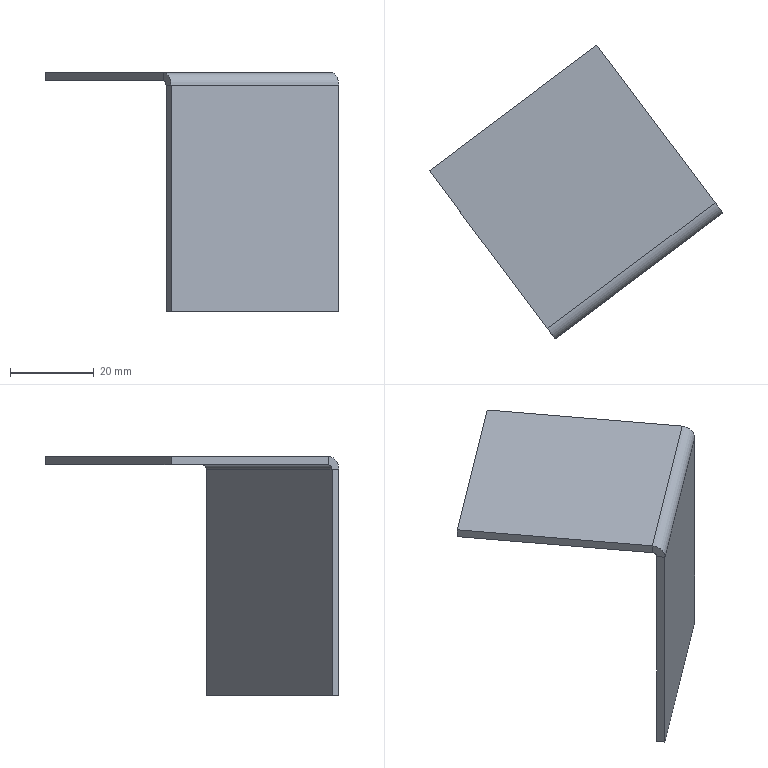Part | SolidWorks | features ICE 5, Split 2, DeleteBody 1, Extrusion 1, FlatPattern 1, SheetMetal 1, Shell 1, SolidToSheetMetal 1 | 1 solid | 14 faces | box 70 x 70 x 57 mm | volume 10414 mm3 | plane 12 | cylinder 2 | commonest cylinder face diameters 2 x1 6 x1
STEP:
#1=CARTESIAN_POINT('',(-960.,255.,4.));
#2=VERTEX_POINT('',#1);
#3=CARTESIAN_POINT('',(-961.2,256.6,4.));
#4=VERTEX_POINT('',#3);
#5=CARTESIAN_POINT('',(-961.2,256.6,4.));
#6=DIRECTION('',(-0.6,0.8,0.));
#7=VECTOR('',#6,1000.);
#8=LINE('',#5,#7);
#9=EDGE_CURVE('',#2,#4,#8,.T.);
#10=ORIENTED_EDGE('',*,*,#9,.F.);
#11=CARTESIAN_POINT('',(-960.,255.,-50.));
#12=VERTEX_POINT('',#11);
#13=CARTESIAN_POINT('',(-960.,255.,0.));
#14=DIRECTION('',(0.,0.,-1.));
#15=VECTOR('',#14,1000.);
#16=LINE('',#13,#15);
#17=EDGE_CURVE('',#2,#12,#16,.T.);
#18=ORIENTED_EDGE('',*,*,#17,.T.);
#19=CARTESIAN_POINT('',(-961.2,256.6,-50.));
#20=VERTEX_POINT('',#19);
#21=CARTESIAN_POINT('',(-961.2,256.6,-50.));
#22=DIRECTION('',(-0.6,0.8,0.));
#23=VECTOR('',#22,1000.);
#24=LINE('',#21,#23);
#25=EDGE_CURVE('',#12,#20,#24,.T.);
#26=ORIENTED_EDGE('',*,*,#25,.T.);
#27=CARTESIAN_POINT('',(-961.2,256.6,-50.));
#28=DIRECTION('',(0.,0.,-1.));
#29=VECTOR('',#28,1000.);
#30=LINE('',#27,#29);
#31=EDGE_CURVE('',#4,#20,#30,.T.);
#32=ORIENTED_EDGE('',*,*,#31,.F.);
#33=EDGE_LOOP('',(#10,#18,#26,#32));
#34=FACE_OUTER_BOUND('',#33,.T.);
#35=CARTESIAN_POINT('',(-961.2,256.6,-50.));
#36=DIRECTION('',(0.8,0.6,0.));
#37=DIRECTION('',(0.,0.,-1.));
#38=AXIS2_PLACEMENT_3D('',#35,#36,#37);
#39=PLANE('',#38);
#40=ADVANCED_FACE('',(#34),#39,.T.);
#41=ORIENTED_EDGE('',*,*,#25,.F.);
#42=CARTESIAN_POINT('',(-1000.,225.,-50.));
#43=VERTEX_POINT('',#42);
#44=CARTESIAN_POINT('',(-468.,624.,-50.));
#45=DIRECTION('',(-0.8,-0.6,0.));
#46=VECTOR('',#45,1000.);
#47=LINE('',#44,#46);
#48=EDGE_CURVE('',#12,#43,#47,.T.);
#49=ORIENTED_EDGE('',*,*,#48,.T.);
#50=CARTESIAN_POINT('',(-1001.2,226.6,-50.));
#51=VERTEX_POINT('',#50);
#52=CARTESIAN_POINT('',(-1001.2,226.6,-50.));
#53=DIRECTION('',(-0.6,0.8,0.));
#54=VECTOR('',#53,1000.);
#55=LINE('',#52,#54);
#56=EDGE_CURVE('',#43,#51,#55,.T.);
#57=ORIENTED_EDGE('',*,*,#56,.T.);
#58=CARTESIAN_POINT('',(-1001.2,226.6,-50.));
#59=DIRECTION('',(-0.8,-0.6,0.));
#60=VECTOR('',#59,1000.);
#61=LINE('',#58,#60);
#62=EDGE_CURVE('',#20,#51,#61,.T.);
#63=ORIENTED_EDGE('',*,*,#62,.F.);
#64=EDGE_LOOP('',(#41,#49,#57,#63));
#65=FACE_OUTER_BOUND('',#64,.T.);
#66=CARTESIAN_POINT('',(-1001.2,226.6,-50.));
#67=DIRECTION('',(0.,0.,-1.));
#68=DIRECTION('',(-0.8,-0.6,0.));
#69=AXIS2_PLACEMENT_3D('',#66,#67,#68);
#70=PLANE('',#69);
#71=ADVANCED_FACE('',(#65),#70,.T.);
#72=ORIENTED_EDGE('',*,*,#56,.F.);
#73=CARTESIAN_POINT('',(-1000.,225.,4.));
#74=VERTEX_POINT('',#73);
#75=CARTESIAN_POINT('',(-1000.,225.,0.));
#76=DIRECTION('',(0.,0.,1.));
#77=VECTOR('',#76,1000.);
#78=LINE('',#75,#77);
#79=EDGE_CURVE('',#43,#74,#78,.T.);
#80=ORIENTED_EDGE('',*,*,#79,.T.);
#81=CARTESIAN_POINT('',(-1001.2,226.6,4.));
#82=VERTEX_POINT('',#81);
#83=CARTESIAN_POINT('',(-1001.2,226.6,4.));
#84=DIRECTION('',(-0.6,0.8,0.));
#85=VECTOR('',#84,1000.);
#86=LINE('',#83,#85);
#87=EDGE_CURVE('',#74,#82,#86,.T.);
#88=ORIENTED_EDGE('',*,*,#87,.T.);
#89=CARTESIAN_POINT('',(-1001.2,226.6,-50.));
#90=DIRECTION('',(0.,0.,1.));
#91=VECTOR('',#90,1000.);
#92=LINE('',#89,#91);
#93=EDGE_CURVE('',#51,#82,#92,.T.);
#94=ORIENTED_EDGE('',*,*,#93,.F.);
#95=EDGE_LOOP('',(#72,#80,#88,#94));
#96=FACE_OUTER_BOUND('',#95,.T.);
#97=CARTESIAN_POINT('',(-1001.2,226.6,-50.));
#98=DIRECTION('',(-0.8,-0.6,0.));
#99=DIRECTION('',(0.,0.,1.));
#100=AXIS2_PLACEMENT_3D('',#97,#98,#99);
#101=PLANE('',#100);
#102=ADVANCED_FACE('',(#96),#101,.T.);
#103=ORIENTED_EDGE('',*,*,#87,.F.);
#104=CARTESIAN_POINT('',(-1001.8,227.4,7.));
#105=VERTEX_POINT('',#104);
#106=CARTESIAN_POINT('',(-1001.8,227.4,4.));
#107=DIRECTION('',(-0.8,-0.6,0.));
#108=DIRECTION('',(0.6,-0.8,0.));
#109=AXIS2_PLACEMENT_3D('',#106,#107,#108);
#110=CIRCLE('',#109,3.);
#111=EDGE_CURVE('',#74,#105,#110,.T.);
#112=ORIENTED_EDGE('',*,*,#111,.T.);
#113=CARTESIAN_POINT('',(-1001.8,227.4,5.));
#114=VERTEX_POINT('',#113);
#115=CARTESIAN_POINT('',(-1001.8,227.4,5.));
#116=DIRECTION('',(0.,0.,-1.));
#117=VECTOR('',#116,1000.);
#118=LINE('',#115,#117);
#119=EDGE_CURVE('',#105,#114,#118,.T.);
#120=ORIENTED_EDGE('',*,*,#119,.T.);
#121=CARTESIAN_POINT('',(-1001.8,227.4,4.));
#122=DIRECTION('',(-0.8,-0.6,0.));
#123=DIRECTION('',(0.6,-0.8,0.));
#124=AXIS2_PLACEMENT_3D('',#121,#122,#123);
#125=CIRCLE('',#124,1.);
#126=EDGE_CURVE('',#82,#114,#125,.T.);
#127=ORIENTED_EDGE('',*,*,#126,.F.);
#128=EDGE_LOOP('',(#103,#112,#120,#127));
#129=FACE_OUTER_BOUND('',#128,.T.);
#130=CARTESIAN_POINT('',(-1001.8,227.4,4.));
#131=DIRECTION('',(0.8,0.6,0.));
#132=DIRECTION('',(-0.6,0.8,0.));
#133=AXIS2_PLACEMENT_3D('',#130,#131,#132);
#134=PLANE('',#133);
#135=ADVANCED_FACE('',(#129),#134,.F.);
#136=ORIENTED_EDGE('',*,*,#119,.F.);
#137=CARTESIAN_POINT('',(-1030.,265.,7.));
#138=VERTEX_POINT('',#137);
#139=CARTESIAN_POINT('',(-1000.,225.,7.));
#140=DIRECTION('',(0.6,-0.8,0.));
#141=VECTOR('',#140,1000.);
#142=LINE('',#139,#141);
#143=EDGE_CURVE('',#138,#105,#142,.T.);
#144=ORIENTED_EDGE('',*,*,#143,.F.);
#145=CARTESIAN_POINT('',(-1030.,265.,5.));
#146=VERTEX_POINT('',#145);
#147=CARTESIAN_POINT('',(-1030.,265.,5.));
#148=DIRECTION('',(0.,0.,-1.));
#149=VECTOR('',#148,1000.);
#150=LINE('',#147,#149);
#151=EDGE_CURVE('',#138,#146,#150,.T.);
#152=ORIENTED_EDGE('',*,*,#151,.T.);
#153=CARTESIAN_POINT('',(-1000.,225.,5.));
#154=DIRECTION('',(0.6,-0.8,0.));
#155=VECTOR('',#154,1000.);
#156=LINE('',#153,#155);
#157=EDGE_CURVE('',#146,#114,#156,.T.);
#158=ORIENTED_EDGE('',*,*,#157,.T.);
#159=EDGE_LOOP('',(#136,#144,#152,#158));
#160=FACE_OUTER_BOUND('',#159,.T.);
#161=CARTESIAN_POINT('',(-1000.,225.,5.));
#162=DIRECTION('',(0.8,0.6,0.));
#163=DIRECTION('',(0.6,-0.8,0.));
#164=AXIS2_PLACEMENT_3D('',#161,#162,#163);
#165=PLANE('',#164);
#166=ADVANCED_FACE('',(#160),#165,.F.);
#167=ORIENTED_EDGE('',*,*,#151,.F.);
#168=CARTESIAN_POINT('',(-990.,295.,7.));
#169=VERTEX_POINT('',#168);
#170=CARTESIAN_POINT('',(-1030.,265.,7.));
#171=DIRECTION('',(-0.8,-0.6,0.));
#172=VECTOR('',#171,1000.);
#173=LINE('',#170,#172);
#174=EDGE_CURVE('',#169,#138,#173,.T.);
#175=ORIENTED_EDGE('',*,*,#174,.F.);
#176=CARTESIAN_POINT('',(-990.,295.,5.));
#177=VERTEX_POINT('',#176);
#178=CARTESIAN_POINT('',(-990.,295.,5.));
#179=DIRECTION('',(0.,0.,-1.));
#180=VECTOR('',#179,1000.);
#181=LINE('',#178,#180);
#182=EDGE_CURVE('',#169,#177,#181,.T.);
#183=ORIENTED_EDGE('',*,*,#182,.T.);
#184=CARTESIAN_POINT('',(-1030.,265.,5.));
#185=DIRECTION('',(-0.8,-0.6,0.));
#186=VECTOR('',#185,1000.);
#187=LINE('',#184,#186);
#188=EDGE_CURVE('',#177,#146,#187,.T.);
#189=ORIENTED_EDGE('',*,*,#188,.T.);
#190=EDGE_LOOP('',(#167,#175,#183,#189));
#191=FACE_OUTER_BOUND('',#190,.T.);
#192=CARTESIAN_POINT('',(-1030.,265.,5.));
#193=DIRECTION('',(0.6,-0.8,0.));
#194=DIRECTION('',(-0.8,-0.6,0.));
#195=AXIS2_PLACEMENT_3D('',#192,#193,#194);
#196=PLANE('',#195);
#197=ADVANCED_FACE('',(#191),#196,.F.);
#198=ORIENTED_EDGE('',*,*,#182,.F.);
#199=CARTESIAN_POINT('',(-961.8,257.4,7.));
#200=VERTEX_POINT('',#199);
#201=CARTESIAN_POINT('',(-990.,295.,7.));
#202=DIRECTION('',(-0.6,0.8,0.));
#203=VECTOR('',#202,1000.);
#204=LINE('',#201,#203);
#205=EDGE_CURVE('',#200,#169,#204,.T.);
#206=ORIENTED_EDGE('',*,*,#205,.F.);
#207=CARTESIAN_POINT('',(-961.8,257.4,5.));
#208=VERTEX_POINT('',#207);
#209=CARTESIAN_POINT('',(-961.8,257.4,5.));
#210=DIRECTION('',(0.,0.,-1.));
#211=VECTOR('',#210,1000.);
#212=LINE('',#209,#211);
#213=EDGE_CURVE('',#200,#208,#212,.T.);
#214=ORIENTED_EDGE('',*,*,#213,.T.);
#215=CARTESIAN_POINT('',(-990.,295.,5.));
#216=DIRECTION('',(-0.6,0.8,0.));
#217=VECTOR('',#216,1000.);
#218=LINE('',#215,#217);
#219=EDGE_CURVE('',#208,#177,#218,.T.);
#220=ORIENTED_EDGE('',*,*,#219,.T.);
#221=EDGE_LOOP('',(#198,#206,#214,#220));
#222=FACE_OUTER_BOUND('',#221,.T.);
#223=CARTESIAN_POINT('',(-990.,295.,5.));
#224=DIRECTION('',(-0.8,-0.6,0.));
#225=DIRECTION('',(-0.6,0.8,0.));
#226=AXIS2_PLACEMENT_3D('',#223,#224,#225);
#227=PLANE('',#226);
#228=ADVANCED_FACE('',(#222),#227,.F.);
#229=CARTESIAN_POINT('',(-961.8,257.4,4.));
#230=DIRECTION('',(0.8,0.6,0.));
#231=DIRECTION('',(0.6,-0.8,0.));
#232=AXIS2_PLACEMENT_3D('',#229,#230,#231);
#233=CIRCLE('',#232,3.);
#234=EDGE_CURVE('',#200,#2,#233,.T.);
#235=ORIENTED_EDGE('',*,*,#234,.T.);
#236=ORIENTED_EDGE('',*,*,#9,.T.);
#237=CARTESIAN_POINT('',(-961.8,257.4,4.));
#238=DIRECTION('',(0.8,0.6,0.));
#239=DIRECTION('',(-0.6,0.8,0.));
#240=AXIS2_PLACEMENT_3D('',#237,#238,#239);
#241=CIRCLE('',#240,1.);
#242=EDGE_CURVE('',#208,#4,#241,.T.);
#243=ORIENTED_EDGE('',*,*,#242,.F.);
#244=ORIENTED_EDGE('',*,*,#213,.F.);
#245=EDGE_LOOP('',(#235,#236,#243,#244));
#246=FACE_OUTER_BOUND('',#245,.T.);
#247=CARTESIAN_POINT('',(-961.8,257.4,4.));
#248=DIRECTION('',(-0.8,-0.6,0.));
#249=DIRECTION('',(0.6,-0.8,0.));
#250=AXIS2_PLACEMENT_3D('',#247,#248,#249);
#251=PLANE('',#250);
#252=ADVANCED_FACE('',(#246),#251,.F.);
#253=ORIENTED_EDGE('',*,*,#219,.F.);
#254=CARTESIAN_POINT('',(-1001.8,227.4,5.));
#255=DIRECTION('',(-0.8,-0.6,0.));
#256=VECTOR('',#255,1000.);
#257=LINE('',#254,#256);
#258=EDGE_CURVE('',#208,#114,#257,.T.);
#259=ORIENTED_EDGE('',*,*,#258,.T.);
#260=ORIENTED_EDGE('',*,*,#157,.F.);
#261=ORIENTED_EDGE('',*,*,#188,.F.);
#262=EDGE_LOOP('',(#253,#259,#260,#261));
#263=FACE_OUTER_BOUND('',#262,.T.);
#264=CARTESIAN_POINT('',(0.,0.,5.));
#265=DIRECTION('',(0.,0.,-1.));
#266=DIRECTION('',(-1.,0.,0.));
#267=AXIS2_PLACEMENT_3D('',#264,#265,#266);
#268=PLANE('',#267);
#269=ADVANCED_FACE('',(#263),#268,.T.);
#270=ORIENTED_EDGE('',*,*,#93,.T.);
#271=CARTESIAN_POINT('',(-961.2,256.6,4.));
#272=DIRECTION('',(0.8,0.6,0.));
#273=VECTOR('',#272,1000.);
#274=LINE('',#271,#273);
#275=EDGE_CURVE('',#82,#4,#274,.T.);
#276=ORIENTED_EDGE('',*,*,#275,.T.);
#277=ORIENTED_EDGE('',*,*,#31,.T.);
#278=ORIENTED_EDGE('',*,*,#62,.T.);
#279=EDGE_LOOP('',(#270,#276,#277,#278));
#280=FACE_OUTER_BOUND('',#279,.T.);
#281=CARTESIAN_POINT('',(-469.2,625.6,0.));
#282=DIRECTION('',(-0.6,0.8,0.));
#283=DIRECTION('',(-0.8,-0.6,0.));
#284=AXIS2_PLACEMENT_3D('',#281,#282,#283);
#285=PLANE('',#284);
#286=ADVANCED_FACE('',(#280),#285,.T.);
#287=ORIENTED_EDGE('',*,*,#126,.T.);
#288=ORIENTED_EDGE('',*,*,#258,.F.);
#289=ORIENTED_EDGE('',*,*,#242,.T.);
#290=ORIENTED_EDGE('',*,*,#275,.F.);
#291=EDGE_LOOP('',(#287,#288,#289,#290));
#292=FACE_OUTER_BOUND('',#291,.T.);
#293=CARTESIAN_POINT('',(-469.8,626.4,4.));
#294=DIRECTION('',(-0.8,-0.6,0.));
#295=DIRECTION('',(0.6,-0.8,0.));
#296=AXIS2_PLACEMENT_3D('',#293,#294,#295);
#297=CYLINDRICAL_SURFACE('',#296,1.);
#298=ADVANCED_FACE('',(#292),#297,.F.);
#299=ORIENTED_EDGE('',*,*,#205,.T.);
#300=ORIENTED_EDGE('',*,*,#174,.T.);
#301=ORIENTED_EDGE('',*,*,#143,.T.);
#302=CARTESIAN_POINT('',(-469.8,626.4,7.));
#303=DIRECTION('',(-0.8,-0.6,0.));
#304=VECTOR('',#303,1000.);
#305=LINE('',#302,#304);
#306=EDGE_CURVE('',#200,#105,#305,.T.);
#307=ORIENTED_EDGE('',*,*,#306,.F.);
#308=EDGE_LOOP('',(#299,#300,#301,#307));
#309=FACE_OUTER_BOUND('',#308,.T.);
#310=CARTESIAN_POINT('',(0.,0.,7.));
#311=DIRECTION('',(0.,0.,-1.));
#312=DIRECTION('',(-1.,0.,0.));
#313=AXIS2_PLACEMENT_3D('',#310,#311,#312);
#314=PLANE('',#313);
#315=ADVANCED_FACE('',(#309),#314,.F.);
#316=ORIENTED_EDGE('',*,*,#79,.F.);
#317=ORIENTED_EDGE('',*,*,#48,.F.);
#318=ORIENTED_EDGE('',*,*,#17,.F.);
#319=CARTESIAN_POINT('',(-468.,624.,4.));
#320=DIRECTION('',(0.8,0.6,0.));
#321=VECTOR('',#320,1000.);
#322=LINE('',#319,#321);
#323=EDGE_CURVE('',#74,#2,#322,.T.);
#324=ORIENTED_EDGE('',*,*,#323,.F.);
#325=EDGE_LOOP('',(#316,#317,#318,#324));
#326=FACE_OUTER_BOUND('',#325,.T.);
#327=CARTESIAN_POINT('',(-468.,624.,0.));
#328=DIRECTION('',(-0.6,0.8,0.));
#329=DIRECTION('',(-0.8,-0.6,0.));
#330=AXIS2_PLACEMENT_3D('',#327,#328,#329);
#331=PLANE('',#330);
#332=ADVANCED_FACE('',(#326),#331,.F.);
#333=ORIENTED_EDGE('',*,*,#111,.F.);
#334=ORIENTED_EDGE('',*,*,#323,.T.);
#335=ORIENTED_EDGE('',*,*,#234,.F.);
#336=ORIENTED_EDGE('',*,*,#306,.T.);
#337=EDGE_LOOP('',(#333,#334,#335,#336));
#338=FACE_OUTER_BOUND('',#337,.T.);
#339=CARTESIAN_POINT('',(-469.8,626.4,4.));
#340=DIRECTION('',(-0.8,-0.6,0.));
#341=DIRECTION('',(0.6,-0.8,0.));
#342=AXIS2_PLACEMENT_3D('',#339,#340,#341);
#343=CYLINDRICAL_SURFACE('',#342,3.);
#344=ADVANCED_FACE('',(#338),#343,.T.);
#345=CLOSED_SHELL('',(#40,#71,#102,#135,#166,#197,#228,#252,#269,#286,#298,#315,#332,#344));
#346=MANIFOLD_SOLID_BREP('',#345);
#347=CARTESIAN_POINT('',(0.,0.,0.));
#348=DIRECTION('',(0.,0.,1.));
#349=DIRECTION('',(1.,0.,0.));
#350=AXIS2_PLACEMENT_3D('',#347,#348,#349);
#351=(LENGTH_UNIT()NAMED_UNIT(*)SI_UNIT(.MILLI.,.METRE.));
#352=UNCERTAINTY_MEASURE_WITH_UNIT(LENGTH_MEASURE(0.00001),#351,'','');
#353=(NAMED_UNIT(*)PLANE_ANGLE_UNIT()SI_UNIT($,.RADIAN.));
#354=(NAMED_UNIT(*)SI_UNIT($,.STERADIAN.)SOLID_ANGLE_UNIT());
#355=(GEOMETRIC_REPRESENTATION_CONTEXT(3)GLOBAL_UNCERTAINTY_ASSIGNED_CONTEXT((#352))GLOBAL_UNIT_ASSIGNED_CONTEXT((#351,#353,#354))REPRESENTATION_CONTEXT('',''));
#356=ADVANCED_BREP_SHAPE_REPRESENTATION('',(#346,#350),#355);